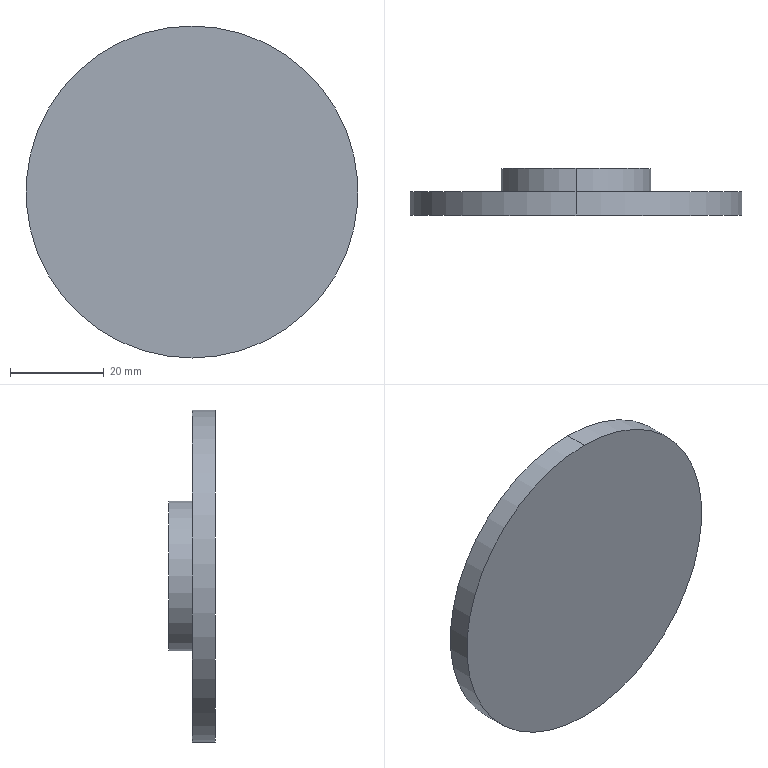Part | SolidWorks | features Extrusion 1, ICE 1 | 1 solid | 7 faces | box 71 x 10 x 71 mm | volume 23815 mm3 | cylinder 4 | plane 3 | commonest cylinder face diameters 31.992 x2 71 x2
STEP:
#1=CARTESIAN_POINT('',(0.,10.,15.996));
#2=VERTEX_POINT('',#1);
#3=CARTESIAN_POINT('',(0.,10.,-15.996));
#4=VERTEX_POINT('',#3);
#5=CARTESIAN_POINT('',(0.,10.,0.));
#6=DIRECTION('',(0.,1.,0.));
#7=DIRECTION('',(0.,0.,1.));
#8=AXIS2_PLACEMENT_3D('',#5,#6,#7);
#9=CIRCLE('',#8,15.996);
#10=EDGE_CURVE('',#2,#4,#9,.T.);
#11=ORIENTED_EDGE('',*,*,#10,.F.);
#12=CARTESIAN_POINT('',(0.,5.,15.996));
#13=VERTEX_POINT('',#12);
#14=CARTESIAN_POINT('',(0.,10.,15.996));
#15=DIRECTION('',(0.,-1.,0.));
#16=VECTOR('',#15,1000.);
#17=LINE('',#14,#16);
#18=EDGE_CURVE('',#2,#13,#17,.T.);
#19=ORIENTED_EDGE('',*,*,#18,.T.);
#20=CARTESIAN_POINT('',(0.,5.,-15.996));
#21=VERTEX_POINT('',#20);
#22=CARTESIAN_POINT('',(0.,5.,0.));
#23=DIRECTION('',(0.,1.,0.));
#24=DIRECTION('',(0.,0.,1.));
#25=AXIS2_PLACEMENT_3D('',#22,#23,#24);
#26=CIRCLE('',#25,15.996);
#27=EDGE_CURVE('',#13,#21,#26,.T.);
#28=ORIENTED_EDGE('',*,*,#27,.T.);
#29=CARTESIAN_POINT('',(0.,10.,-15.996));
#30=DIRECTION('',(0.,-1.,0.));
#31=VECTOR('',#30,1000.);
#32=LINE('',#29,#31);
#33=EDGE_CURVE('',#4,#21,#32,.T.);
#34=ORIENTED_EDGE('',*,*,#33,.F.);
#35=EDGE_LOOP('',(#11,#19,#28,#34));
#36=FACE_OUTER_BOUND('',#35,.T.);
#37=CARTESIAN_POINT('',(0.,10.,0.));
#38=DIRECTION('',(0.,-1.,0.));
#39=DIRECTION('',(0.,0.,-1.));
#40=AXIS2_PLACEMENT_3D('',#37,#38,#39);
#41=CYLINDRICAL_SURFACE('',#40,15.996);
#42=ADVANCED_FACE('',(#36),#41,.T.);
#43=CARTESIAN_POINT('',(0.,5.,35.5));
#44=VERTEX_POINT('',#43);
#45=CARTESIAN_POINT('',(0.,5.,-35.5));
#46=VERTEX_POINT('',#45);
#47=CARTESIAN_POINT('',(0.,5.,0.));
#48=DIRECTION('',(0.,1.,0.));
#49=DIRECTION('',(0.,0.,1.));
#50=AXIS2_PLACEMENT_3D('',#47,#48,#49);
#51=CIRCLE('',#50,35.5);
#52=EDGE_CURVE('',#44,#46,#51,.T.);
#53=ORIENTED_EDGE('',*,*,#52,.F.);
#54=CARTESIAN_POINT('',(0.,0.,35.5));
#55=VERTEX_POINT('',#54);
#56=CARTESIAN_POINT('',(0.,5.,35.5));
#57=DIRECTION('',(0.,-1.,0.));
#58=VECTOR('',#57,1000.);
#59=LINE('',#56,#58);
#60=EDGE_CURVE('',#44,#55,#59,.T.);
#61=ORIENTED_EDGE('',*,*,#60,.T.);
#62=CARTESIAN_POINT('',(0.,0.,-35.5));
#63=VERTEX_POINT('',#62);
#64=CARTESIAN_POINT('',(0.,0.,0.));
#65=DIRECTION('',(0.,1.,0.));
#66=DIRECTION('',(0.,0.,1.));
#67=AXIS2_PLACEMENT_3D('',#64,#65,#66);
#68=CIRCLE('',#67,35.5);
#69=EDGE_CURVE('',#55,#63,#68,.T.);
#70=ORIENTED_EDGE('',*,*,#69,.T.);
#71=CARTESIAN_POINT('',(0.,5.,-35.5));
#72=DIRECTION('',(0.,-1.,0.));
#73=VECTOR('',#72,1000.);
#74=LINE('',#71,#73);
#75=EDGE_CURVE('',#46,#63,#74,.T.);
#76=ORIENTED_EDGE('',*,*,#75,.F.);
#77=EDGE_LOOP('',(#53,#61,#70,#76));
#78=FACE_OUTER_BOUND('',#77,.T.);
#79=CARTESIAN_POINT('',(0.,5.,0.));
#80=DIRECTION('',(0.,-1.,0.));
#81=DIRECTION('',(0.,0.,-1.));
#82=AXIS2_PLACEMENT_3D('',#79,#80,#81);
#83=CYLINDRICAL_SURFACE('',#82,35.5);
#84=ADVANCED_FACE('',(#78),#83,.T.);
#85=ORIENTED_EDGE('',*,*,#60,.F.);
#86=CARTESIAN_POINT('',(0.,5.,0.));
#87=DIRECTION('',(0.,1.,0.));
#88=DIRECTION('',(0.,0.,1.));
#89=AXIS2_PLACEMENT_3D('',#86,#87,#88);
#90=CIRCLE('',#89,35.5);
#91=EDGE_CURVE('',#46,#44,#90,.T.);
#92=ORIENTED_EDGE('',*,*,#91,.F.);
#93=ORIENTED_EDGE('',*,*,#75,.T.);
#94=CARTESIAN_POINT('',(0.,0.,0.));
#95=DIRECTION('',(0.,1.,0.));
#96=DIRECTION('',(0.,0.,1.));
#97=AXIS2_PLACEMENT_3D('',#94,#95,#96);
#98=CIRCLE('',#97,35.5);
#99=EDGE_CURVE('',#63,#55,#98,.T.);
#100=ORIENTED_EDGE('',*,*,#99,.T.);
#101=EDGE_LOOP('',(#85,#92,#93,#100));
#102=FACE_OUTER_BOUND('',#101,.T.);
#103=CARTESIAN_POINT('',(0.,5.,0.));
#104=DIRECTION('',(0.,-1.,0.));
#105=DIRECTION('',(0.,0.,-1.));
#106=AXIS2_PLACEMENT_3D('',#103,#104,#105);
#107=CYLINDRICAL_SURFACE('',#106,35.5);
#108=ADVANCED_FACE('',(#102),#107,.T.);
#109=CARTESIAN_POINT('',(0.,5.,0.));
#110=DIRECTION('',(0.,1.,0.));
#111=DIRECTION('',(0.,0.,1.));
#112=AXIS2_PLACEMENT_3D('',#109,#110,#111);
#113=CIRCLE('',#112,15.996);
#114=EDGE_CURVE('',#21,#13,#113,.T.);
#115=ORIENTED_EDGE('',*,*,#114,.F.);
#116=ORIENTED_EDGE('',*,*,#27,.F.);
#117=EDGE_LOOP('',(#115,#116));
#118=FACE_BOUND('',#117,.T.);
#119=ORIENTED_EDGE('',*,*,#91,.T.);
#120=ORIENTED_EDGE('',*,*,#52,.T.);
#121=EDGE_LOOP('',(#119,#120));
#122=FACE_OUTER_BOUND('',#121,.T.);
#123=CARTESIAN_POINT('',(0.,5.,0.));
#124=DIRECTION('',(0.,1.,0.));
#125=DIRECTION('',(0.,0.,1.));
#126=AXIS2_PLACEMENT_3D('',#123,#124,#125);
#127=PLANE('',#126);
#128=ADVANCED_FACE('',(#118,#122),#127,.T.);
#129=ORIENTED_EDGE('',*,*,#99,.F.);
#130=ORIENTED_EDGE('',*,*,#69,.F.);
#131=EDGE_LOOP('',(#129,#130));
#132=FACE_OUTER_BOUND('',#131,.T.);
#133=CARTESIAN_POINT('',(0.,0.,0.));
#134=DIRECTION('',(0.,1.,0.));
#135=DIRECTION('',(0.,0.,1.));
#136=AXIS2_PLACEMENT_3D('',#133,#134,#135);
#137=PLANE('',#136);
#138=ADVANCED_FACE('',(#132),#137,.F.);
#139=ORIENTED_EDGE('',*,*,#18,.F.);
#140=CARTESIAN_POINT('',(0.,10.,0.));
#141=DIRECTION('',(0.,1.,0.));
#142=DIRECTION('',(0.,0.,1.));
#143=AXIS2_PLACEMENT_3D('',#140,#141,#142);
#144=CIRCLE('',#143,15.996);
#145=EDGE_CURVE('',#4,#2,#144,.T.);
#146=ORIENTED_EDGE('',*,*,#145,.F.);
#147=ORIENTED_EDGE('',*,*,#33,.T.);
#148=ORIENTED_EDGE('',*,*,#114,.T.);
#149=EDGE_LOOP('',(#139,#146,#147,#148));
#150=FACE_OUTER_BOUND('',#149,.T.);
#151=CARTESIAN_POINT('',(0.,10.,0.));
#152=DIRECTION('',(0.,-1.,0.));
#153=DIRECTION('',(0.,0.,-1.));
#154=AXIS2_PLACEMENT_3D('',#151,#152,#153);
#155=CYLINDRICAL_SURFACE('',#154,15.996);
#156=ADVANCED_FACE('',(#150),#155,.T.);
#157=ORIENTED_EDGE('',*,*,#145,.T.);
#158=ORIENTED_EDGE('',*,*,#10,.T.);
#159=EDGE_LOOP('',(#157,#158));
#160=FACE_OUTER_BOUND('',#159,.T.);
#161=CARTESIAN_POINT('',(0.,10.,0.));
#162=DIRECTION('',(0.,1.,0.));
#163=DIRECTION('',(0.,0.,1.));
#164=AXIS2_PLACEMENT_3D('',#161,#162,#163);
#165=PLANE('',#164);
#166=ADVANCED_FACE('',(#160),#165,.T.);
#167=CLOSED_SHELL('',(#42,#84,#108,#128,#138,#156,#166));
#168=MANIFOLD_SOLID_BREP('',#167);
#169=CARTESIAN_POINT('',(0.,0.,0.));
#170=DIRECTION('',(0.,0.,1.));
#171=DIRECTION('',(1.,0.,0.));
#172=AXIS2_PLACEMENT_3D('',#169,#170,#171);
#173=(LENGTH_UNIT()NAMED_UNIT(*)SI_UNIT(.MILLI.,.METRE.));
#174=UNCERTAINTY_MEASURE_WITH_UNIT(LENGTH_MEASURE(0.00001),#173,'','');
#175=(NAMED_UNIT(*)PLANE_ANGLE_UNIT()SI_UNIT($,.RADIAN.));
#176=(NAMED_UNIT(*)SI_UNIT($,.STERADIAN.)SOLID_ANGLE_UNIT());
#177=(GEOMETRIC_REPRESENTATION_CONTEXT(3)GLOBAL_UNCERTAINTY_ASSIGNED_CONTEXT((#174))GLOBAL_UNIT_ASSIGNED_CONTEXT((#173,#175,#176))REPRESENTATION_CONTEXT('',''));
#178=ADVANCED_BREP_SHAPE_REPRESENTATION('',(#168,#172),#177);